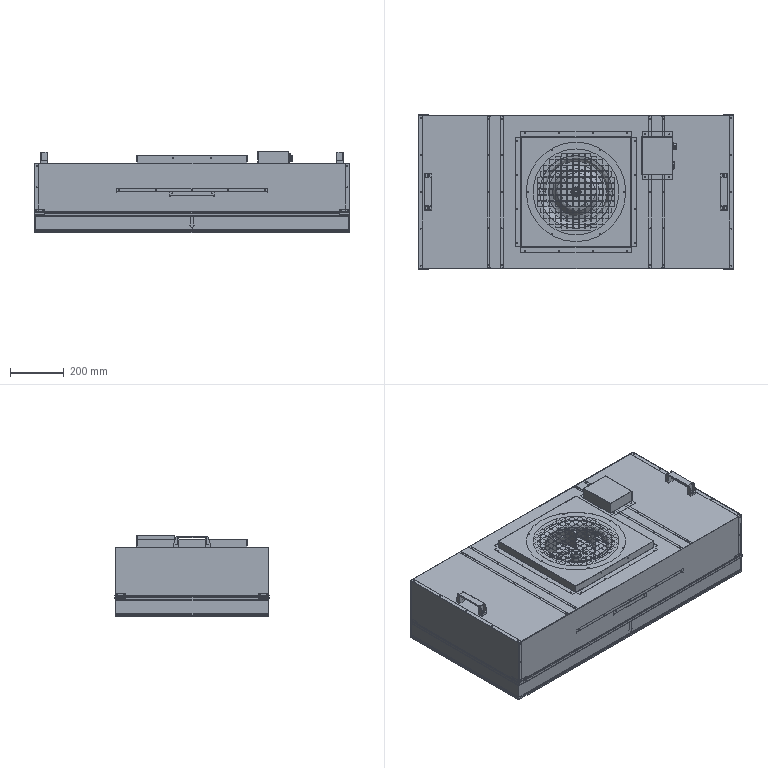Part | SolidWorks | 27 solids | 2665 faces | box 1174 x 574 x 303.9 mm | volume 75861290 mm3 | plane 1499 | cylinder 847 | spline 288 | cone 31 | commonest cylinder face diameters 3.5 x352 1 x88 0.4 x68 1.6 x68 10 x41 6 x36